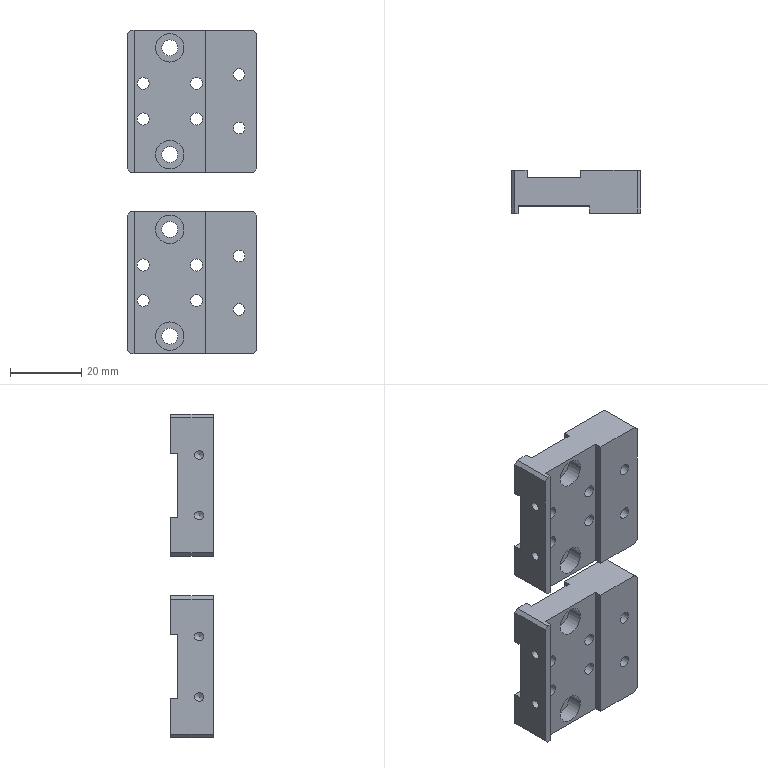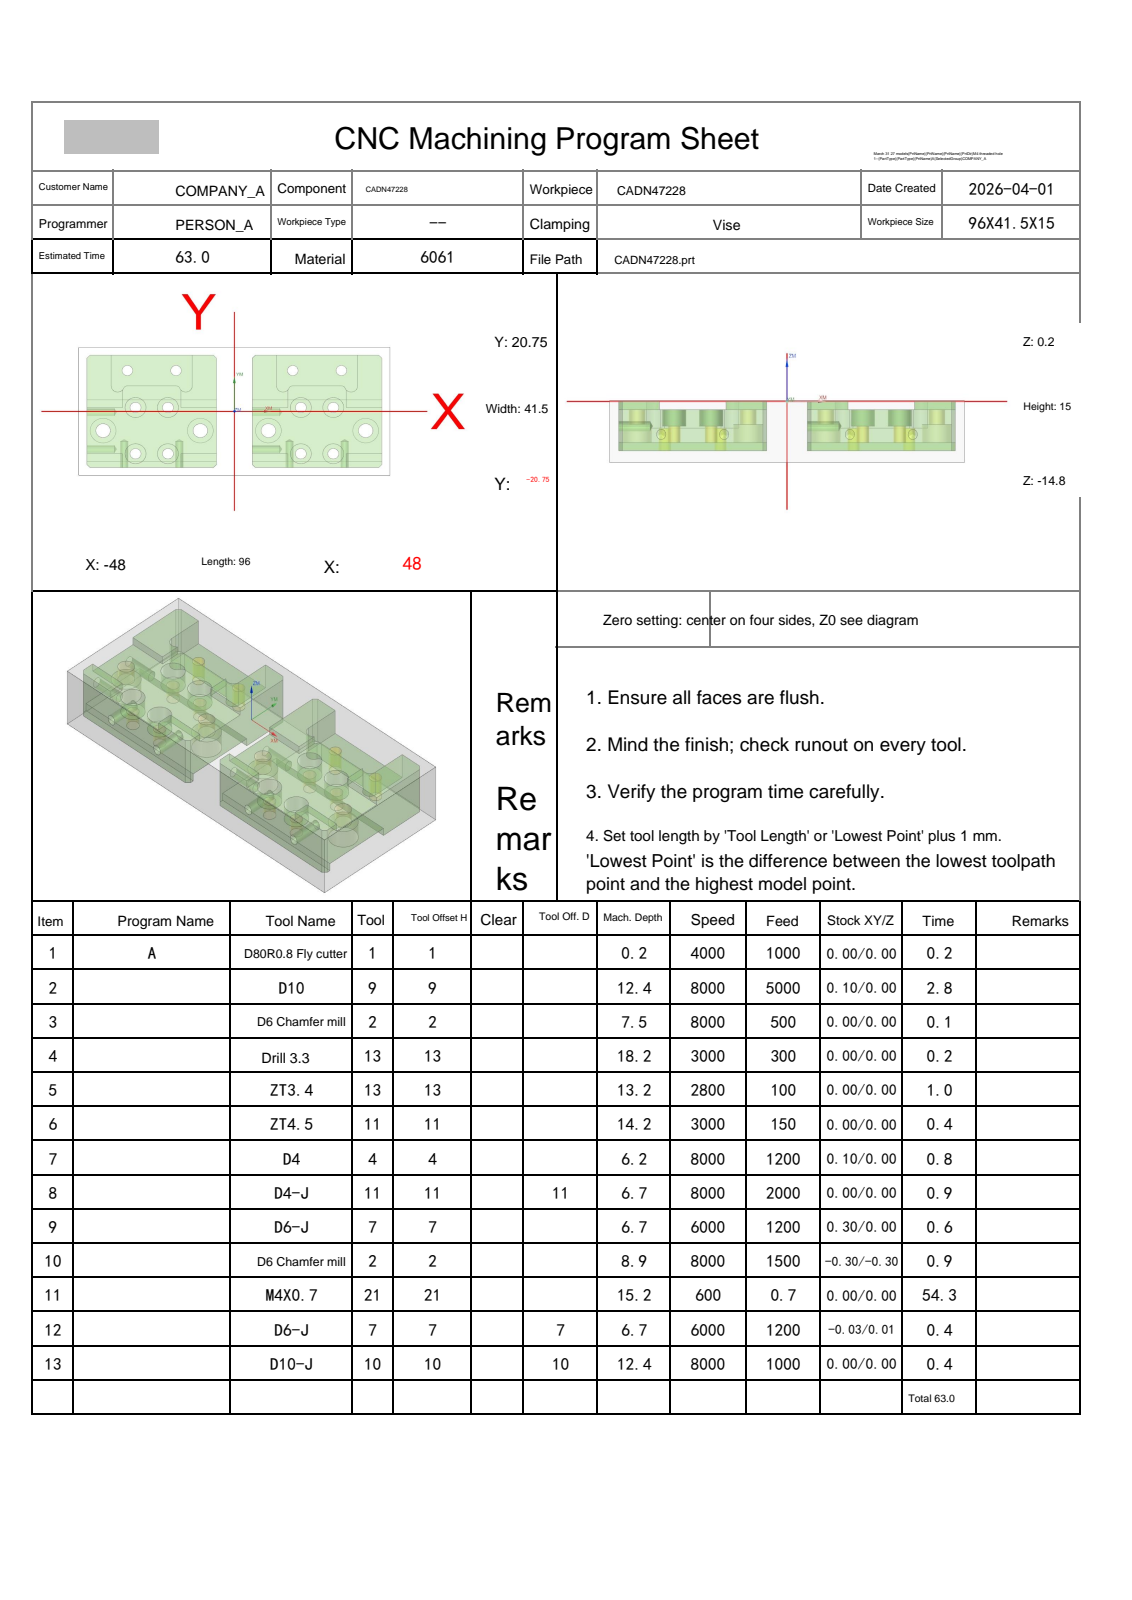NC program | NX | posted by the shop | part box 36.5 x 12 x 91 mm
Lines 4409 to 5439 of 5439:
N9 T07 M06
(D6-J  D=6. R=0. H=07 ce=0.30 di=0.00)
G00 G90 G54 X25.5 Y-24.25 M03 S6000
G43 H07 Z20.
M08
Z-1.5
G01 Z-2. F1200.
Y-18.85
X19.8
Y-10.45
X4.9
Y-2.05
X19.8
Y6.927
G03 X19.182 Y8.85 I-3.3 J0.0
G01 X31.818
G03 X31.2 Y6.927 I2.682 J-1.923
G01 Y-2.05
X46.1
Y-10.45
X31.2
Y-18.85
X25.5
Y-14.65
X24.
Y-10.45
G03 X19.8 Y-6.25 I-4.2 J0.0
G01 X9.1
X19.8
G03 X24. Y-2.05 I0.0 J4.2
G01 Y4.65
X27.
Y-2.05
G03 X31.2 Y-6.25 I4.2 J0.0
G01 X41.9
X31.2
G03 X27.73 Y-8.083 I0.0 J-4.2
G01 X25.5 Y-6.562
G03 X25.274 Y-6.25 I-5.7 J-3.888
X25.5 Y-5.938 I-5.474 J4.2
X25.726 Y-6.25 I5.7 J3.888
X25.5 Y-6.562 I5.474 J-4.2
G01 X27.73 Y-8.083
G03 X27. Y-10.45 I3.47 J-2.367
G01 Y-14.65
X25.5
X25.
Y-24.25
Z-1.5
G00 Z20.
X-25.5
Z-1.5
G01 Z-2.
Y-18.85
X-31.2
Y-10.45
X-46.1
Y-2.05
X-31.2
Y6.927
G03 X-31.818 Y8.85 I-3.3 J0.0
G01 X-19.182
G03 X-19.8 Y6.927 I2.682 J-1.923
G01 Y-2.05
X-4.9
Y-10.45
X-19.8
Y-18.85
X-25.5
Y-14.65
X-27.
Y-10.45
G03 X-31.2 Y-6.25 I-4.2 J0.0
G01 X-41.9
X-31.2
G03 X-27. Y-2.05 I0.0 J4.2
G01 Y4.65
X-24.
Y-2.05
G03 X-19.8 Y-6.25 I4.2 J0.0
G01 X-9.1
X-19.8
G03 X-23.27 Y-8.083 I0.0 J-4.2
G01 X-25.5 Y-6.562
G03 X-25.726 Y-6.25 I-5.7 J-3.888
X-25.5 Y-5.938 I-5.474 J4.2
X-25.274 Y-6.25 I5.7 J3.888
X-25.5 Y-6.562 I5.474 J-4.2
G01 X-23.27 Y-8.083
G03 X-24. Y-10.45 I3.47 J-2.367
G01 Y-14.65
X-25.5
X-26.
Y-24.25
Z-1.5
G00 Z20.
G00 G90 X-25.5 Y24.25 M03 S6000
Z20.
Z-6.
G01 Z-6.5 F1200.
Y18.85
X-16.3
Y11.269
G03 X-17.828 Y11.55 I-1.528 J-4.019
G01 X-33.172
G03 X-34.7 Y11.269 I0.0 J-4.3
G01 Y18.85
X-25.5
Y16.15
X-19.
Y14.25
X-32.
Y16.15
X-25.5
X-25.
Y24.25
Z-6.
G00 Z20.
X25.5
Z-6.
G01 Z-6.5
Y18.85
X34.7
Y11.269
G03 X33.172 Y11.55 I-1.528 J-4.019
G01 X17.828
G03 X16.3 Y11.269 I0.0 J-4.3
G01 Y18.85
X25.5
Y16.15
X32.
Y14.25
X19.
Y16.15
X25.5
X26.
Y24.25
Z-6.
G00 Z20.
G91 G28 Z0.0
M05
M09
G91 G28 Z0.0
M01
N10 T02 M06
(D6 Chamfer mill  D=6. R=0. H=02 ce=0.00 di=0.00)
G00 G90 G54 X33. Y13.25 M03 S8000
G43 H02 Z20.
M08
G98 G81 X33. Y13.25 Z-8.7 R-3.5 F500.
X18.
X-18.
X-33.
G80
G00 Z20.
G00 G90 X40.482 Y-5.7 M03 S8000
Z20.
Z-2.5
G01 Z-3. F500.
X40.45 Y-4.75
G03 X38.95 Y-6.25 I0.0 J-1.5
X40.5 Y-7.8 I1.55 J0.0
X42.05 Y-6.25 I0.0 J1.55
X40.5 Y-4.7 I-1.55 J0.0
X38.95 Y-6.25 I0.0 J-1.55
X40.45 Y-7.75 I1.5 J0.0
G01 X40.482 Y-6.8
Z-2.5
G00 Z20.
X10.482 Y-5.7
Z-2.5
G01 Z-3.
X10.45 Y-4.75
G03 X8.95 Y-6.25 I0.0 J-1.5
X10.5 Y-7.8 I1.55 J0.0
X12.05 Y-6.25 I0.0 J1.55
X10.5 Y-4.7 I-1.55 J0.0
X8.95 Y-6.25 I0.0 J-1.55
X10.45 Y-7.75 I1.5 J0.0
G01 X10.482 Y-6.8
Z-2.5
G00 Z20.
X-10.518 Y-5.7
Z-2.5
G01 Z-3.
X-10.55 Y-4.75
G03 X-12.05 Y-6.25 I0.0 J-1.5
X-10.5 Y-7.8 I1.55 J0.0
X-8.95 Y-6.25 I0.0 J1.55
X-10.5 Y-4.7 I-1.55 J0.0
X-12.05 Y-6.25 I0.0 J-1.55
X-10.55 Y-7.75 I1.5 J0.0
G01 X-10.518 Y-6.8
Z-2.5
G00 Z20.
X-40.518 Y-5.7
Z-2.5
G01 Z-3.
X-40.55 Y-4.75
G03 X-42.05 Y-6.25 I0.0 J-1.5
X-40.5 Y-7.8 I1.55 J0.0
X-38.95 Y-6.25 I0.0 J1.55
X-40.5 Y-4.7 I-1.55 J0.0
X-42.05 Y-6.25 I0.0 J-1.55
X-40.55 Y-7.75 I1.5 J0.0
G01 X-40.518 Y-6.8
Z-2.5
G00 Z20.
G00 G90 X39.614 Y-12.523 M03 S6500
Z20.
Z.172
G01 Z-1.2 F1500.
G03 X39.9 Y-12.723 I1.286 J1.532
G01 X39.946 Y-12.753
X40. Y-12.75
X45.5
G02 X46.5 Y-13.75 I0.0 J-1.
G01 Y-17.25
X46.466 Y-17.509
X46.366 Y-17.75
X46.207 Y-17.957
X45.207 Y-18.957
X45. Y-19.116
X44.759 Y-19.216
X44.5 Y-19.25
X34.5
G02 X33.5 Y-18.25 I0.0 J1.
G01 Y-13.75
G02 X34.5 Y-12.75 I1. J0.0
G01 X40.
X40.054 Y-12.753
X40.1 Y-12.723
G03 X40.386 Y-12.523 I-1. J1.732
G01 Z.172
G00 Z10.
X46.727 Y9.636
Z.172
G01 Z-1.2
G03 X46.527 Y9.35 I1.532 J-1.286
G01 X46.497 Y9.304
X46.5 Y9.25
Y1.25
G02 X45.5 Y.25 I-1. J0.0
G01 X34.5
G02 X33.5 Y1.25 I0.0 J1.
G01 Y6.927
G02 X34.5 Y7.927 I1. J0.0
X35.047 Y7.764 I0.0 J-1.
G01 X35.453 Y7.413
G03 X36. Y7.25 I.547 J.837
X37. Y8.25 I0.0 J1.
G01 Y18.25
G02 X38. Y19.25 I1. J0.0
G01 X44.5
X44.759 Y19.216
X45. Y19.116
X45.207 Y18.957
X46.207 Y17.957
X46.366 Y17.75
X46.466 Y17.509
X46.5 Y17.25
Y9.25
X46.497 Y9.196
X46.527 Y9.15
G03 X46.727 Y8.864 I1.732 J1.
G01 Z.172
G00 Z10.
X4.273
Z.172
G01 Z-1.2
G03 X4.473 Y9.15 I-1.532 J1.286
G01 X4.503 Y9.196
X4.5 Y9.25
Y17.25
X4.534 Y17.509
X4.634 Y17.75
X4.793 Y17.957
X5.793 Y18.957
X6. Y19.116
X6.241 Y19.216
X6.5 Y19.25
X13.
G02 X14. Y18.25 I0.0 J-1.
G01 Y8.25
G03 X15. Y7.25 I1. J0.0
X15.547 Y7.413 I0.0 J1.
G01 X15.953 Y7.764
G02 X16.5 Y7.927 I.547 J-.837
X17.5 Y6.927 I0.0 J-1.
G01 Y1.25
G02 X16.5 Y.25 I-1. J0.0
G01 X5.5
G02 X4.5 Y1.25 I0.0 J1.
G01 Y9.25
X4.503 Y9.304
X4.473 Y9.35
G03 X4.273 Y9.636 I-1.732 J-1.
G01 Z.172
G00 Z10.
X10.614 Y-12.523
Z.172
G01 Z-1.2
G03 X10.9 Y-12.723 I1.286 J1.532
G01 X10.946 Y-12.753
X11. Y-12.75
X16.5
G02 X17.5 Y-13.75 I0.0 J-1.
G01 Y-18.25
G02 X16.5 Y-19.25 I-1. J0.0
G01 X6.5
X6.241 Y-19.216
X6. Y-19.116
X5.793 Y-18.957
X4.793 Y-17.957
X4.634 Y-17.75
X4.534 Y-17.509
X4.5 Y-17.25
Y-13.75
G02 X5.5 Y-12.75 I1. J0.0
G01 X11.
X11.054 Y-12.753
X11.1 Y-12.723
G03 X11.386 Y-12.523 I-1. J1.732
G01 Z.172
G00 Z10.
X-11.386
Z.172
G01 Z-1.2
G03 X-11.1 Y-12.723 I1.286 J1.532
G01 X-11.054 Y-12.753
X-11. Y-12.75
X-5.5
G02 X-4.5 Y-13.75 I0.0 J-1.
G01 Y-17.25
X-4.534 Y-17.509
X-4.634 Y-17.75
X-4.793 Y-17.957
X-5.793 Y-18.957
X-6. Y-19.116
X-6.241 Y-19.216
X-6.5 Y-19.25
X-16.5
G02 X-17.5 Y-18.25 I0.0 J1.
G01 Y-13.75
G02 X-16.5 Y-12.75 I1. J0.0
G01 X-11.
X-10.946 Y-12.753
X-10.9 Y-12.723
G03 X-10.614 Y-12.523 I-1. J1.732
G01 Z.172
G00 Z10.
X-4.273 Y9.636
Z.172
G01 Z-1.2
G03 X-4.473 Y9.35 I1.532 J-1.286
G01 X-4.503 Y9.304
X-4.5 Y9.25
Y1.25
G02 X-5.5 Y.25 I-1. J0.0
G01 X-16.5
G02 X-17.5 Y1.25 I0.0 J1.
G01 Y6.927
G02 X-16.5 Y7.927 I1. J0.0
X-15.953 Y7.764 I0.0 J-1.
G01 X-15.547 Y7.413
G03 X-15. Y7.25 I.547 J.837
X-14. Y8.25 I0.0 J1.
G01 Y18.25
G02 X-13. Y19.25 I1. J0.0
G01 X-6.5
X-6.241 Y19.216
X-6. Y19.116
X-5.793 Y18.957
X-4.793 Y17.957
X-4.634 Y17.75
X-4.534 Y17.509
X-4.5 Y17.25
Y9.25
X-4.503 Y9.196
X-4.473 Y9.15
G03 X-4.273 Y8.864 I1.732 J1.
G01 Z.172
G00 Z10.
X-46.727
Z.172
G01 Z-1.2
G03 X-46.527 Y9.15 I-1.532 J1.286
G01 X-46.497 Y9.196
X-46.5 Y9.25
Y17.25
X-46.466 Y17.509
X-46.366 Y17.75
X-46.207 Y17.957
X-45.207 Y18.957
X-45. Y19.116
X-44.759 Y19.216
X-44.5 Y19.25
X-38.
G02 X-37. Y18.25 I0.0 J-1.
G01 Y8.25
G03 X-36. Y7.25 I1. J0.0
X-35.453 Y7.413 I0.0 J1.
G01 X-35.047 Y7.764
G02 X-34.5 Y7.927 I.547 J-.837
X-33.5 Y6.927 I0.0 J-1.
G01 Y1.25
G02 X-34.5 Y.25 I-1. J0.0
G01 X-45.5
G02 X-46.5 Y1.25 I0.0 J1.
G01 Y9.25
X-46.497 Y9.304
X-46.527 Y9.35
G03 X-46.727 Y9.636 I-1.732 J-1.
G01 Z.172
G00 Z10.
X-40.386 Y-12.523
Z.172
G01 Z-1.2
G03 X-40.1 Y-12.723 I1.286 J1.532
G01 X-40.054 Y-12.753
X-40. Y-12.75
X-34.5
G02 X-33.5 Y-13.75 I0.0 J-1.
G01 Y-18.25
G02 X-34.5 Y-19.25 I-1. J0.0
G01 X-44.5
X-44.759 Y-19.216
X-45. Y-19.116
X-45.207 Y-18.957
X-46.207 Y-17.957
X-46.366 Y-17.75
X-46.466 Y-17.509
X-46.5 Y-17.25
Y-13.75
G02 X-45.5 Y-12.75 I1. J0.0
G01 X-40.
X-39.946 Y-12.753
X-39.9 Y-12.723
G03 X-39.614 Y-12.523 I-1. J1.732
G01 Z.172
G00 Z10.
X-4.432 Y-1.74
Z-1.669
G01 Z-3.2
X-4.492 Y-1.825
X-4.5 Y-1.855
Y-10.645
X-4.492 Y-10.675
X-4.432 Y-10.76
Z-1.669
G00 Z10.
X-32.598 Y9.477
Z-1.782
G01 Z-3.2
G03 X-32.313 Y9.277 I1.286 J1.532
G01 X-32.267 Y9.247
X-32.213 Y9.25
X-18.787
X-18.733 Y9.247
X-18.687 Y9.277
G03 X-18.402 Y9.477 I-1. J1.732
G01 Z-1.782
G00 Z10.
X-46.568 Y-10.76
Z-1.669
G01 Z-3.2
X-46.508 Y-10.675
X-46.5 Y-10.645
Y-1.855
X-46.508 Y-1.825
X-46.568 Y-1.74
Z-1.669
G00 Z10.
X-19.478 Y-19.318
Z-1.669
G01 Z-3.2
X-19.564 Y-19.258
X-19.594 Y-19.25
X-31.406
X-31.436 Y-19.258
X-31.522 Y-19.318
Z-1.669
G00 Z10.
X-19.652 Y3.249
Z-1.671
G01 Z-3.2
X-19.687 Y3.311
X-19.742 Y3.356
X-19.754 Y3.378
X-19.778 Y3.377
G03 X-20.504 Y3.498 I-.726 J-2.125
X-22.75 Y1.252 I0.0 J-2.246
X-22.716 Y.859 I2.246 J0.0
X-20.5 Y-1. I2.216 J.391
X-19.375 Y-.699 I0.0 J2.25
G01 X-19.214 Y-.586
X-19.194 Y-.562
X-19.159 Y-.464
Z-1.67
G00 Z10.
X-31.841
Z-1.665
G01 Z-3.2
X-31.806 Y-.562
X-31.786 Y-.586
X-31.625 Y-.699
G03 X-30.5 Y-1. I1.125 J1.949
X-28.25 Y1.25 I0.0 J2.25
G01 Y1.254
G03 X-30.492 Y3.497 I-2.242 J0.0
X-31.247 Y3.366 I0.0 J-2.242
G01 X-31.272 Y3.346
X-31.326 Y3.257
Z-1.674
G00 Z10.
X-41.565 Y-5.843
Z-1.706
G01 Z-3.2
G03 X-41.734 Y-6.148 I1.658 J-1.118
G01 X-41.759 Y-6.196
X-41.75 Y-6.25
G03 X-40.5 Y-7.5 I1.25 J0.0
X-39.25 Y-6.25 I0.0 J1.25
X-40.5 Y-5. I-1.25 J0.0
X-41.723 Y-5.99 I0.0 J-1.25
G01 X-41.75 Y-6.25
X-41.759 Y-6.304
X-41.734 Y-6.352
G03 X-41.565 Y-6.657 I1.827 J.813
G01 Z-1.706
G00 Z10.
X-31.348 Y-15.749
Z-1.673
G01 Z-3.2
X-31.313 Y-15.811
X-31.258 Y-15.856
X-31.246 Y-15.878
X-31.222 Y-15.877
G03 X-30.496 Y-15.998 I.726 J2.125
X-28.25 Y-13.752 I0.0 J2.246
X-28.284 Y-13.359 I-2.246 J0.0
X-30.5 Y-11.5 I-2.216 J-.391
X-31.625 Y-11.801 I0.0 J-2.25
G01 X-31.786 Y-11.914
X-31.806 Y-11.938
X-31.841 Y-12.036
Z-1.665
G00 Z10.
X-19.159
Z-1.67
G01 Z-3.2
X-19.194 Y-11.938
X-19.214 Y-11.914
X-19.375 Y-11.801
G03 X-20.5 Y-11.5 I-1.125 J-1.949
X-22.75 Y-13.75 I0.0 J-2.25
G01 Y-13.754
G03 X-20.508 Y-15.997 I2.242 J0.0
X-19.753 Y-15.866 I0.0 J2.242
G01 X-19.728 Y-15.846
X-19.674 Y-15.757
Z-1.673
G00 Z10.
X-11.565 Y-5.843
Z-1.706
G01 Z-3.2
G03 X-11.734 Y-6.148 I1.658 J-1.118
G01 X-11.759 Y-6.196
X-11.75 Y-6.25
G03 X-10.5 Y-7.5 I1.25 J0.0
X-9.25 Y-6.25 I0.0 J1.25
X-10.5 Y-5. I-1.25 J0.0
X-11.723 Y-5.99 I0.0 J-1.25
G01 X-11.75 Y-6.25
X-11.759 Y-6.304
X-11.734 Y-6.352
G03 X-11.565 Y-6.657 I1.827 J.813
G01 Z-1.706
G00 Z10.
X31.522 Y-19.318
Z-1.669
G01 Z-3.2
X31.436 Y-19.258
X31.406 Y-19.25
X19.594
X19.564 Y-19.258
X19.478 Y-19.318
Z-1.669
G00 Z10.
X46.568 Y-1.74
Z-1.669
G01 Z-3.2
X46.508 Y-1.825
X46.5 Y-1.855
Y-10.645
X46.508 Y-10.675
X46.568 Y-10.76
Z-1.669
G00 Z10.
X18.402 Y9.477
Z-1.782
G01 Z-3.2
G03 X18.687 Y9.277 I1.286 J1.532
G01 X18.733 Y9.247
X18.787 Y9.25
X32.213
X32.267 Y9.247
X32.313 Y9.277
G03 X32.598 Y9.477 I-1. J1.732
G01 Z-1.782
G00 Z10.
X4.432 Y-10.76
Z-1.669
G01 Z-3.2
X4.492 Y-10.675
X4.5 Y-10.645
Y-1.855
X4.492 Y-1.825
X4.432 Y-1.74
Z-1.669
G00 Z10.
X31.348 Y3.249
Z-1.671
G01 Z-3.2
X31.313 Y3.311
X31.258 Y3.356
X31.246 Y3.378
X31.222 Y3.377
G03 X30.496 Y3.498 I-.726 J-2.125
X28.25 Y1.252 I0.0 J-2.246
X28.284 Y.859 I2.246 J0.0
X30.5 Y-1. I2.216 J.391
X31.625 Y-.699 I0.0 J2.25
G01 X31.786 Y-.586
X31.806 Y-.562
X31.841 Y-.464
Z-1.67
G00 Z10.
X19.159
Z-1.665
G01 Z-3.2
X19.194 Y-.562
X19.214 Y-.586
X19.375 Y-.699
G03 X20.5 Y-1. I1.125 J1.949
X22.75 Y1.25 I0.0 J2.25
G01 Y1.254
G03 X20.508 Y3.497 I-2.242 J0.0
X19.753 Y3.366 I0.0 J-2.242
G01 X19.728 Y3.346
X19.674 Y3.257
Z-1.674
G00 Z10.
X9.435 Y-5.843
Z-1.706
G01 Z-3.2
G03 X9.266 Y-6.148 I1.658 J-1.118
G01 X9.241 Y-6.196
X9.25 Y-6.25
G03 X10.5 Y-7.5 I1.25 J0.0
X11.75 Y-6.25 I0.0 J1.25
X10.5 Y-5. I-1.25 J0.0
X9.277 Y-5.99 I0.0 J-1.25
G01 X9.25 Y-6.25
X9.241 Y-6.304
X9.266 Y-6.352
G03 X9.435 Y-6.657 I1.827 J.813
G01 Z-1.706
G00 Z10.
X19.652 Y-15.749
Z-1.673
G01 Z-3.2
X19.687 Y-15.811
X19.742 Y-15.856
X19.754 Y-15.878
X19.778 Y-15.877
G03 X20.504 Y-15.998 I.726 J2.125
X22.75 Y-13.752 I0.0 J2.246
X22.716 Y-13.359 I-2.246 J0.0
X20.5 Y-11.5 I-2.216 J-.391
X19.375 Y-11.801 I0.0 J-2.25
G01 X19.214 Y-11.914
X19.194 Y-11.938
X19.159 Y-12.036
Z-1.665
G00 Z10.
X31.841
Z-1.67
G01 Z-3.2
X31.806 Y-11.938
X31.786 Y-11.914
X31.625 Y-11.801
G03 X30.5 Y-11.5 I-1.125 J-1.949
X28.25 Y-13.75 I0.0 J-2.25
G01 Y-13.754
G03 X30.492 Y-15.997 I2.242 J0.0
X31.247 Y-15.866 I0.0 J2.242
G01 X31.272 Y-15.846
X31.326 Y-15.757
Z-1.673
G00 Z10.
X39.435 Y-5.843
Z-1.706
G01 Z-3.2
G03 X39.266 Y-6.148 I1.658 J-1.118
G01 X39.241 Y-6.196
X39.25 Y-6.25
G03 X40.5 Y-7.5 I1.25 J0.0
X41.75 Y-6.25 I0.0 J1.25
X40.5 Y-5. I-1.25 J0.0
X39.277 Y-5.99 I0.0 J-1.25
G01 X39.25 Y-6.25
X39.241 Y-6.304
X39.266 Y-6.352
G03 X39.435 Y-6.657 I1.827 J.813
G01 Z-1.706
G00 Z10.
X-34.991 Y19.318
Z-1.795
G01 Z-7.7
X-34.905 Y19.258
X-34.875 Y19.25
X-16.125
X-16.095 Y19.258
X-16.009 Y19.318
Z-1.795
G00 Z10.
X-32.506 Y12.831
Z-6.095
G01 Z-7.7
G03 X-32.359 Y13.147 I-1.732 J1.
G01 X-32.338 Y13.197
X-32.35 Y13.25
G03 X-33. Y13.9 I-.65 J0.0
X-33.65 Y13.25 I0.0 J-.65
X-33. Y12.6 I.65 J0.0
X-32.35 Y13.25 I0.0 J.65
G01 X-32.338 Y13.303
X-32.359 Y13.353
G03 X-32.506 Y13.669 I-1.879 J-.684
G01 Z-6.095
G00 Z10.
X-17.506 Y12.831
Z-6.095
G01 Z-7.7
G03 X-17.359 Y13.147 I-1.732 J1.
G01 X-17.338 Y13.197
X-17.35 Y13.25
G03 X-18. Y13.9 I-.65 J0.0
X-18.65 Y13.25 I0.0 J-.65
X-18. Y12.6 I.65 J0.0
X-17.35 Y13.25 I0.0 J.65
G01 X-17.338 Y13.303
X-17.359 Y13.353
G03 X-17.506 Y13.669 I-1.879 J-.684
G01 Z-6.095
G00 Z10.
X16.009 Y19.318
Z-1.795
G01 Z-7.7
X16.095 Y19.258
X16.125 Y19.25
X34.875
X34.905 Y19.258
X34.991 Y19.318
Z-1.795
G00 Z10.
X18.494 Y12.831
Z-6.095
G01 Z-7.7
G03 X18.641 Y13.147 I-1.732 J1.
G01 X18.662 Y13.197
X18.65 Y13.25
G03 X18. Y13.9 I-.65 J0.0
X17.35 Y13.25 I0.0 J-.65
X18. Y12.6 I.65 J0.0
X18.65 Y13.25 I0.0 J.65
G01 X18.662 Y13.303
X18.641 Y13.353
G03 X18.494 Y13.669 I-1.879 J-.684
G01 Z-6.095
G00 Z10.
X33.494 Y12.831
Z-6.095
G01 Z-7.7
G03 X33.641 Y13.147 I-1.732 J1.
G01 X33.662 Y13.197
X33.65 Y13.25
G03 X33. Y13.9 I-.65 J0.0
X32.35 Y13.25 I0.0 J-.65
X33. Y12.6 I.65 J0.0
X33.65 Y13.25 I0.0 J.65
G01 X33.662 Y13.303
X33.641 Y13.353
G03 X33.494 Y13.669 I-1.879 J-.684
G01 Z-6.095
G00 Z20.
G91 G28 Z0.0
M05
M09
G91 G28 Z0.0
M01
N11 T21 M06
(M4X0.7 D=3.3 DR_a=180 H=21)
G00 G90 G54 X33. Y13.25 M03 S600
G43 H21 Z20.
M08
G95
G98 G84 X33. Y13.25 Z-15. R-5.5 F.7 Q4.
X18.
X-18.
X-33.
G80
G94
G00 Z20.
G91 G28 Z0.0
M05
M09
G91 G28 Z0.0
M01
N12 T07 M06
(D6-J  D=6. R=0. H=07 ce=-0.03 di=0.01)
G00 G90 G54 X17.07 Y11.449 M03 S6000
G43 H07 Z20.
M08
Z-1.495
G01 Z-1.995 F1200.
G41 D07
X16.97
G03 X15.97 Y10.449 I0.0 J-1.
G01 Y9.849
G02 X16.5 Y9.897 I.53 J-2.922
X19.47 Y6.927 I0.0 J-2.97
G01 Y-1.72
X2.8
G03 X1.8 Y-2.72 I0.0 J-1.
G01 G40 Y-2.82
Z-1.495
G00 Z20.
Y-9.68
Z-1.495
G01 Z-1.995
G41 D07
Y-9.78
G03 X2.8 Y-10.78 I1. J0.0
G01 X19.47
Y-20.95
G03 X20.47 Y-21.95 I1. J0.0
G01 G40 X20.57
Z-1.495
G00 Z20.
X30.43
Z-1.495
G01 Z-1.995
G41 D07
X30.53
G03 X31.53 Y-20.95 I0.0 J1.
G01 Y-10.78
X48.2
G03 X49.2 Y-9.78 I0.0 J1.
G01 G40 Y-9.68
Z-1.495
G00 Z20.
Y-2.82
Z-1.495
G01 Z-1.995
G41 D07
Y-2.72
G03 X48.2 Y-1.72 I-1. J0.0
G01 X31.53
Y6.927
G02 X34.5 Y9.897 I2.97 J0.0
X35.03 Y9.849 I0.0 J-2.97
G01 Y10.449
G03 X34.03 Y11.449 I-1. J0.0
G01 G40 X33.93
Z-1.495
G00 Z20.
X-1.8 Y-2.82
Z-1.495
G01 Z-1.995
G41 D07
Y-2.72
G03 X-2.8 Y-1.72 I-1. J0.0
G01 X-19.47
Y6.927
G02 X-16.5 Y9.897 I2.97 J0.0
X-15.97 Y9.849 I0.0 J-2.97
G01 Y10.449
G03 X-16.97 Y11.449 I-1. J0.0
G01 G40 X-17.07
Z-1.495
G00 Z20.
X-33.93
Z-1.495
G01 Z-1.995
G41 D07
X-34.03
G03 X-35.03 Y10.449 I0.0 J-1.
G01 Y9.849
G02 X-34.5 Y9.897 I.53 J-2.922
X-31.53 Y6.927 I0.0 J-2.97
G01 Y-1.72
X-48.2
G03 X-49.2 Y-2.72 I0.0 J-1.
G01 G40 Y-2.82
Z-1.495
G00 Z20.
Y-9.68
Z-1.495
G01 Z-1.995
G41 D07
Y-9.78
G03 X-48.2 Y-10.78 I1. J0.0
G01 X-31.53
Y-20.95
G03 X-30.53 Y-21.95 I1. J0.0
G01 G40 X-30.43
Z-1.495
G00 Z20.
X-20.57
Z-1.495
G01 Z-1.995
G41 D07
X-20.47
G03 X-19.47 Y-20.95 I0.0 J1.
G01 Y-10.78
X-2.8
G03 X-1.8 Y-9.78 I0.0 J1.
G01 G40 Y-9.68
Z-1.495
G00 Z20.
G00 G90 X-33.93 Y21.95 M03 S6000
Z20.
Z-5.995
G01 Z-6.495 F1200.
G41 D07
X-34.03
G03 X-35.03 Y20.95 I0.0 J-1.
G01 Y10.758
G02 X-33.172 Y11.22 I1.858 J-3.508
G01 X-17.828
G02 X-15.97 Y10.758 I0.0 J-3.97
G01 Y20.95
G03 X-16.97 Y21.95 I-1. J0.0
G01 G40 X-17.07
Z-5.995
G00 Z20.
X17.07
Z-5.995
G01 Z-6.495
G41 D07
X16.97
G03 X15.97 Y20.95 I0.0 J-1.
G01 Y10.758
G02 X17.828 Y11.22 I1.858 J-3.508
G01 X33.172
G02 X35.03 Y10.758 I0.0 J-3.97
G01 Y20.95
G03 X34.03 Y21.95 I-1. J0.0
G01 G40 X33.93
Z-5.995
G00 Z20.
G91 G28 Z0.0
M05
M09
G91 G28 Z0.0
M01
N13 T10 M06
(D10-J  D=10. R=0. H=10 ce=0.00 di=0.00)
G00 G90 G54 X-5.487 Y-24.366 M03 S8000
G43 H10 Z20.
M08
Z-11.7
G01 Z-12.2 F1000.
G41 D10
X-5.503 Y-24.167
G03 X-6.5 Y-23.25 I-.997 J-.083
G01 X-44.5
G02 X-48.036 Y-21.786 I0.0 J5.
G01 X-49.036 Y-20.786
G02 X-50.5 Y-17.25 I3.536 J3.536
G01 Y17.25
G02 X-49.036 Y20.786 I5. J0.0
G01 X-48.036 Y21.786
G02 X-44.5 Y23.25 I3.536 J-3.536
G01 X-6.5
G02 X-2.964 Y21.786 I0.0 J-5.
G01 X-1.964 Y20.786
G02 X-.5 Y17.25 I-3.536 J-3.536
G01 Y-17.25
G02 X-1.964 Y-20.786 I-5. J0.0
G01 X-2.964 Y-21.786
G02 X-6.5 Y-23.25 I-3.536 J3.536
G01 X-7.
G03 X-8. Y-24.25 I0.0 J-1.
G01 G40 Y-24.45
X.483 Y-20.891
G41 D10
X.654 Y-20.787
G03 X1.133 Y-19.933 I-.52 J.854
X1.028 Y-19.486 I-1. J0.0
G02 X.5 Y-17.25 I4.472 J2.236
G01 Y17.25
G02 X1.964 Y20.786 I5. J0.0
G01 X2.964 Y21.786
G02 X6.5 Y23.25 I3.536 J-3.536
G01 X44.5
G02 X48.036 Y21.786 I0.0 J-5.
G01 X49.036 Y20.786
G02 X50.5 Y17.25 I-3.536 J-3.536
G01 Y-17.25
G02 X49.036 Y-20.786 I-5. J0.0
G01 X48.036 Y-21.786
G02 X44.5 Y-23.25 I-3.536 J3.536
G01 X6.5
G02 X2.964 Y-21.786 I0.0 J5.
G01 X1.964 Y-20.786
G02 X1.028 Y-19.486 I3.536 J3.536
X.827 Y-19.028 I4.472 J2.236
G03 X-.108 Y-18.384 I-.935 J-.356
X-.463 Y-18.45 I0.0 J-1.
G01 G40 X0.0 Y-19.648
Z-11.7
G00 Z20.
M05
M09
G91 G28 Z0.0
G91 G28 Y0.0
M30
%